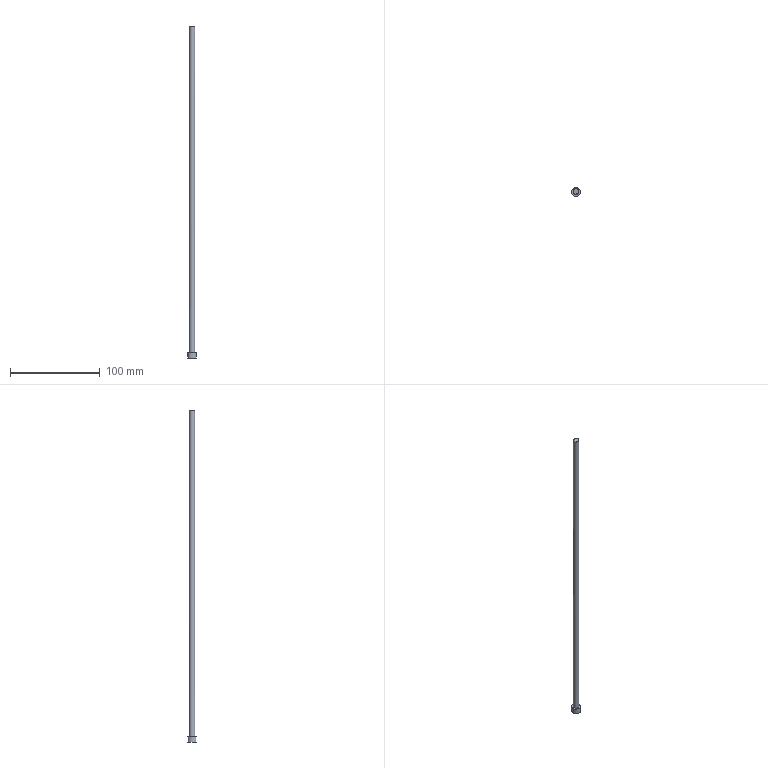Part | NX | features solid 2 | 1 solid | 5 faces | box 10 x 10 x 369.226 mm | volume 10724 mm3 | cylinder 2 | plane 2 | spline 1 | commonest cylinder face diameters 6 x1 10 x1
STEP:
#1=CARTESIAN_POINT('',(26.5,31.,-339.5));
#2=VERTEX_POINT('',#1);
#3=CARTESIAN_POINT('',(29.5,31.,-339.5));
#4=DIRECTION('',(0.,0.,1.));
#5=DIRECTION('',(-1.,0.,0.));
#6=AXIS2_PLACEMENT_3D('',#3,#4,#5);
#7=CIRCLE('',#6,3.);
#8=EDGE_CURVE('',#2,#2,#7,.T.);
#9=ORIENTED_EDGE('',*,*,#8,.T.);
#10=EDGE_LOOP('',(#9));
#11=FACE_BOUND('',#10,.T.);
#12=CARTESIAN_POINT('',(26.516,30.694,22.699));
#13=VERTEX_POINT('',#12);
#14=CARTESIAN_POINT('',(27.415,28.414,22.894));
#15=CARTESIAN_POINT('',(26.186,30.658,22.639));
#16=CARTESIAN_POINT('',(26.935,33.118,22.741));
#17=CARTESIAN_POINT('',(29.169,34.301,23.119));
#18=CARTESIAN_POINT('',(31.586,33.586,23.537));
#19=CARTESIAN_POINT('',(32.813,31.343,23.771));
#20=CARTESIAN_POINT('',(32.069,28.885,23.684));
#21=CARTESIAN_POINT('',(29.827,27.698,23.325));
#22=CARTESIAN_POINT('',(27.415,28.414,22.894));
#23=CARTESIAN_POINT('',(26.186,30.658,22.639));
#24=CARTESIAN_POINT('',(26.935,33.118,22.741));
#25=B_SPLINE_CURVE_WITH_KNOTS('',3,(#14,#15,#16,#17,#18,#19,#20,#21,#22,#23,#24),.UNSPECIFIED.,.T.,.F.,(1,1,1,1,1,1,1,1,1,1,1,1,1,1,1),(-0.007087,-0.004725,-0.002362,0.,0.002362,0.004725,0.007087,0.009449,0.01181,0.01417,0.01654,0.0189,0.02126,0.02362,0.02599),.UNSPECIFIED.);
#26=EDGE_CURVE('',#13,#13,#25,.T.);
#27=ORIENTED_EDGE('',*,*,#26,.T.);
#28=EDGE_LOOP('',(#27));
#29=FACE_BOUND('',#28,.T.);
#30=CARTESIAN_POINT('',(29.5,31.,-345.5));
#31=DIRECTION('',(0.,0.,1.));
#32=DIRECTION('',(-1.,0.,0.));
#33=AXIS2_PLACEMENT_3D('',#30,#31,#32);
#34=CYLINDRICAL_SURFACE('',#33,3.);
#35=ADVANCED_FACE('',(#11,#29),#34,.T.);
#36=ORIENTED_EDGE('',*,*,#8,.F.);
#37=EDGE_LOOP('',(#36));
#38=FACE_BOUND('',#37,.T.);
#39=CARTESIAN_POINT('',(24.5,31.,-339.5));
#40=VERTEX_POINT('',#39);
#41=CARTESIAN_POINT('',(29.5,31.,-339.5));
#42=DIRECTION('',(0.,0.,-1.));
#43=DIRECTION('',(-1.,0.,0.));
#44=AXIS2_PLACEMENT_3D('',#41,#42,#43);
#45=CIRCLE('',#44,5.);
#46=EDGE_CURVE('',#40,#40,#45,.T.);
#47=ORIENTED_EDGE('',*,*,#46,.F.);
#48=EDGE_LOOP('',(#47));
#49=FACE_BOUND('',#48,.T.);
#50=CARTESIAN_POINT('',(29.5,31.,-339.5));
#51=DIRECTION('',(0.,0.,1.));
#52=DIRECTION('',(-1.,0.,0.));
#53=AXIS2_PLACEMENT_3D('',#50,#51,#52);
#54=PLANE('',#53);
#55=ADVANCED_FACE('',(#38,#49),#54,.T.);
#56=CARTESIAN_POINT('',(24.5,31.,-345.5));
#57=VERTEX_POINT('',#56);
#58=CARTESIAN_POINT('',(29.5,31.,-345.5));
#59=DIRECTION('',(0.,0.,1.));
#60=DIRECTION('',(-1.,0.,0.));
#61=AXIS2_PLACEMENT_3D('',#58,#59,#60);
#62=CIRCLE('',#61,5.);
#63=EDGE_CURVE('',#57,#57,#62,.T.);
#64=ORIENTED_EDGE('',*,*,#63,.F.);
#65=EDGE_LOOP('',(#64));
#66=FACE_BOUND('',#65,.T.);
#67=CARTESIAN_POINT('',(29.5,31.,-345.5));
#68=DIRECTION('',(0.,0.,-1.));
#69=DIRECTION('',(1.,0.,0.));
#70=AXIS2_PLACEMENT_3D('',#67,#68,#69);
#71=PLANE('',#70);
#72=ADVANCED_FACE('',(#66),#71,.T.);
#73=ORIENTED_EDGE('',*,*,#46,.T.);
#74=EDGE_LOOP('',(#73));
#75=FACE_BOUND('',#74,.T.);
#76=ORIENTED_EDGE('',*,*,#63,.T.);
#77=EDGE_LOOP('',(#76));
#78=FACE_BOUND('',#77,.T.);
#79=CARTESIAN_POINT('',(29.5,31.,-345.5));
#80=DIRECTION('',(0.,0.,1.));
#81=DIRECTION('',(-1.,0.,0.));
#82=AXIS2_PLACEMENT_3D('',#79,#80,#81);
#83=CYLINDRICAL_SURFACE('',#82,5.);
#84=ADVANCED_FACE('',(#75,#78),#83,.T.);
#85=ORIENTED_EDGE('',*,*,#26,.F.);
#86=EDGE_LOOP('',(#85));
#87=FACE_BOUND('',#86,.T.);
#88=CARTESIAN_POINT('',(26.442,27.945,22.723));
#89=CARTESIAN_POINT('',(26.444,29.976,22.696));
#90=CARTESIAN_POINT('',(26.447,32.007,22.668));
#91=CARTESIAN_POINT('',(26.45,34.038,22.638));
#92=CARTESIAN_POINT('',(28.474,27.945,23.091));
#93=CARTESIAN_POINT('',(28.476,29.976,23.064));
#94=CARTESIAN_POINT('',(28.479,32.007,23.036));
#95=CARTESIAN_POINT('',(28.482,34.038,23.006));
#96=CARTESIAN_POINT('',(30.511,27.945,23.44));
#97=CARTESIAN_POINT('',(30.513,29.976,23.413));
#98=CARTESIAN_POINT('',(30.515,32.006,23.385));
#99=CARTESIAN_POINT('',(30.518,34.038,23.355));
#100=CARTESIAN_POINT('',(32.551,27.945,23.775));
#101=CARTESIAN_POINT('',(32.553,29.975,23.748));
#102=CARTESIAN_POINT('',(32.556,32.006,23.719));
#103=CARTESIAN_POINT('',(32.558,34.037,23.69));
#104=B_SPLINE_SURFACE_WITH_KNOTS('',3,3,((#88,#89,#90,#91),(#92,#93,#94,#95),(#96,#97,#98,#99),(#100,#101,#102,#103)),.UNSPECIFIED.,.F.,.F.,.F.,(4,4),(4,4),(0.7831,0.8142),(0.08225,0.1979),.PIECEWISE_BEZIER_KNOTS.);
#105=ADVANCED_FACE('',(#87),#104,.T.);
#106=CLOSED_SHELL('',(#35,#55,#72,#84,#105));
#107=MANIFOLD_SOLID_BREP('',#106);
#108=(LENGTH_UNIT()NAMED_UNIT(*)SI_UNIT(.MILLI.,.METRE.));
#109=UNCERTAINTY_MEASURE_WITH_UNIT(LENGTH_MEASURE(0.0508),#108,'','');
#110=(NAMED_UNIT(*)PLANE_ANGLE_UNIT()SI_UNIT($,.RADIAN.));
#111=(NAMED_UNIT(*)SI_UNIT($,.STERADIAN.)SOLID_ANGLE_UNIT());
#112=(GEOMETRIC_REPRESENTATION_CONTEXT(3)GLOBAL_UNCERTAINTY_ASSIGNED_CONTEXT((#109))GLOBAL_UNIT_ASSIGNED_CONTEXT((#108,#110,#111))REPRESENTATION_CONTEXT('',''));
#113=ADVANCED_BREP_SHAPE_REPRESENTATION('',(#107),#112);